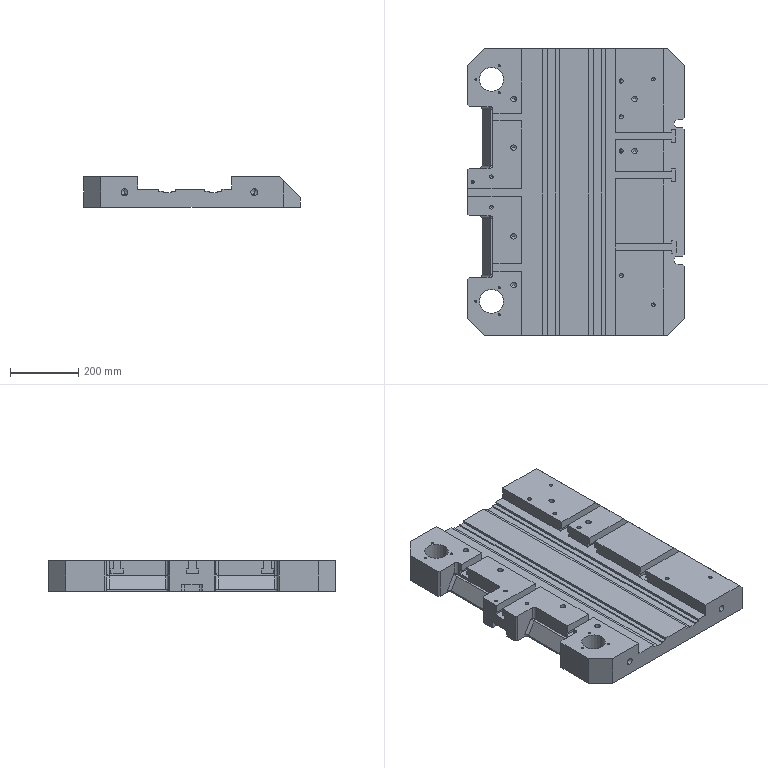Part | 1 solid | 251 faces | box 635 x 840 x 89.05 mm | volume 32535154 mm3 | plane 114 | cylinder 80 | cone 54 | spline 3 | commonest cylinder face diameters 16 x30 6 x12 8 x10 10 x8 12 x8 20 x8